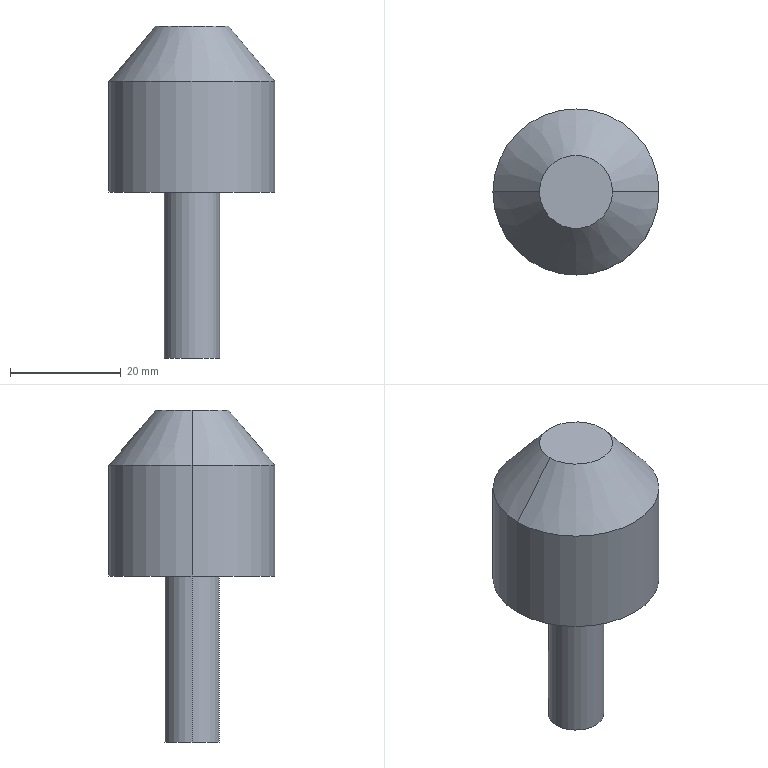Part | SolidWorks | features Chamfer 1, Extrusion 1, ICE 1 | 1 solid | 9 faces | box 30 x 30 x 60 mm | volume 20345 mm3 | cylinder 4 | plane 3 | cone 2 | commonest cylinder face diameters 10 x2 30 x2
STEP:
#1=CARTESIAN_POINT('',(6.609,0.,60.));
#2=VERTEX_POINT('',#1);
#3=CARTESIAN_POINT('',(-6.609,0.,60.));
#4=VERTEX_POINT('',#3);
#5=CARTESIAN_POINT('',(0.,0.,60.));
#6=DIRECTION('',(0.,0.,1.));
#7=DIRECTION('',(1.,0.,0.));
#8=AXIS2_PLACEMENT_3D('',#5,#6,#7);
#9=CIRCLE('',#8,6.609);
#10=EDGE_CURVE('',#2,#4,#9,.T.);
#11=ORIENTED_EDGE('',*,*,#10,.F.);
#12=CARTESIAN_POINT('',(15.,0.,50.));
#13=VERTEX_POINT('',#12);
#14=CARTESIAN_POINT('',(6.609,0.,60.));
#15=DIRECTION('',(0.6428,0.,-0.766));
#16=VECTOR('',#15,1000.);
#17=LINE('',#14,#16);
#18=EDGE_CURVE('',#2,#13,#17,.T.);
#19=ORIENTED_EDGE('',*,*,#18,.T.);
#20=CARTESIAN_POINT('',(-15.,0.,50.));
#21=VERTEX_POINT('',#20);
#22=CARTESIAN_POINT('',(0.,0.,50.));
#23=DIRECTION('',(0.,0.,-1.));
#24=DIRECTION('',(1.,0.,0.));
#25=AXIS2_PLACEMENT_3D('',#22,#23,#24);
#26=CIRCLE('',#25,15.);
#27=EDGE_CURVE('',#21,#13,#26,.T.);
#28=ORIENTED_EDGE('',*,*,#27,.F.);
#29=CARTESIAN_POINT('',(-6.609,0.,60.));
#30=DIRECTION('',(-0.6428,0.,-0.766));
#31=VECTOR('',#30,1000.);
#32=LINE('',#29,#31);
#33=EDGE_CURVE('',#4,#21,#32,.T.);
#34=ORIENTED_EDGE('',*,*,#33,.F.);
#35=EDGE_LOOP('',(#11,#19,#28,#34));
#36=FACE_OUTER_BOUND('',#35,.T.);
#37=CARTESIAN_POINT('',(0.,0.,60.));
#38=DIRECTION('',(0.,0.,-1.));
#39=DIRECTION('',(-1.,0.,0.));
#40=AXIS2_PLACEMENT_3D('',#37,#38,#39);
#41=CONICAL_SURFACE('',#40,6.609,0.6981);
#42=ADVANCED_FACE('',(#36),#41,.T.);
#43=ORIENTED_EDGE('',*,*,#27,.T.);
#44=CARTESIAN_POINT('',(15.,0.,30.));
#45=VERTEX_POINT('',#44);
#46=CARTESIAN_POINT('',(15.,0.,60.));
#47=DIRECTION('',(0.,0.,-1.));
#48=VECTOR('',#47,1000.);
#49=LINE('',#46,#48);
#50=EDGE_CURVE('',#13,#45,#49,.T.);
#51=ORIENTED_EDGE('',*,*,#50,.T.);
#52=CARTESIAN_POINT('',(-15.,0.,30.));
#53=VERTEX_POINT('',#52);
#54=CARTESIAN_POINT('',(0.,0.,30.));
#55=DIRECTION('',(0.,0.,1.));
#56=DIRECTION('',(1.,0.,0.));
#57=AXIS2_PLACEMENT_3D('',#54,#55,#56);
#58=CIRCLE('',#57,15.);
#59=EDGE_CURVE('',#45,#53,#58,.T.);
#60=ORIENTED_EDGE('',*,*,#59,.T.);
#61=CARTESIAN_POINT('',(-15.,0.,60.));
#62=DIRECTION('',(0.,0.,-1.));
#63=VECTOR('',#62,1000.);
#64=LINE('',#61,#63);
#65=EDGE_CURVE('',#21,#53,#64,.T.);
#66=ORIENTED_EDGE('',*,*,#65,.F.);
#67=EDGE_LOOP('',(#43,#51,#60,#66));
#68=FACE_OUTER_BOUND('',#67,.T.);
#69=CARTESIAN_POINT('',(0.,0.,60.));
#70=DIRECTION('',(0.,0.,-1.));
#71=DIRECTION('',(-1.,0.,0.));
#72=AXIS2_PLACEMENT_3D('',#69,#70,#71);
#73=CYLINDRICAL_SURFACE('',#72,15.);
#74=ADVANCED_FACE('',(#68),#73,.T.);
#75=CARTESIAN_POINT('',(5.,0.,30.));
#76=VERTEX_POINT('',#75);
#77=CARTESIAN_POINT('',(-5.,0.,30.));
#78=VERTEX_POINT('',#77);
#79=CARTESIAN_POINT('',(0.,0.,30.));
#80=DIRECTION('',(0.,0.,1.));
#81=DIRECTION('',(1.,0.,0.));
#82=AXIS2_PLACEMENT_3D('',#79,#80,#81);
#83=CIRCLE('',#82,5.);
#84=EDGE_CURVE('',#76,#78,#83,.T.);
#85=ORIENTED_EDGE('',*,*,#84,.F.);
#86=CARTESIAN_POINT('',(5.,0.,0.));
#87=VERTEX_POINT('',#86);
#88=CARTESIAN_POINT('',(5.,0.,30.));
#89=DIRECTION('',(0.,0.,-1.));
#90=VECTOR('',#89,1000.);
#91=LINE('',#88,#90);
#92=EDGE_CURVE('',#76,#87,#91,.T.);
#93=ORIENTED_EDGE('',*,*,#92,.T.);
#94=CARTESIAN_POINT('',(-5.,0.,0.));
#95=VERTEX_POINT('',#94);
#96=CARTESIAN_POINT('',(0.,0.,0.));
#97=DIRECTION('',(0.,0.,1.));
#98=DIRECTION('',(1.,0.,0.));
#99=AXIS2_PLACEMENT_3D('',#96,#97,#98);
#100=CIRCLE('',#99,5.);
#101=EDGE_CURVE('',#87,#95,#100,.T.);
#102=ORIENTED_EDGE('',*,*,#101,.T.);
#103=CARTESIAN_POINT('',(-5.,0.,30.));
#104=DIRECTION('',(0.,0.,-1.));
#105=VECTOR('',#104,1000.);
#106=LINE('',#103,#105);
#107=EDGE_CURVE('',#78,#95,#106,.T.);
#108=ORIENTED_EDGE('',*,*,#107,.F.);
#109=EDGE_LOOP('',(#85,#93,#102,#108));
#110=FACE_OUTER_BOUND('',#109,.T.);
#111=CARTESIAN_POINT('',(0.,0.,30.));
#112=DIRECTION('',(0.,0.,-1.));
#113=DIRECTION('',(-1.,0.,0.));
#114=AXIS2_PLACEMENT_3D('',#111,#112,#113);
#115=CYLINDRICAL_SURFACE('',#114,5.);
#116=ADVANCED_FACE('',(#110),#115,.T.);
#117=ORIENTED_EDGE('',*,*,#92,.F.);
#118=CARTESIAN_POINT('',(0.,0.,30.));
#119=DIRECTION('',(0.,0.,1.));
#120=DIRECTION('',(1.,0.,0.));
#121=AXIS2_PLACEMENT_3D('',#118,#119,#120);
#122=CIRCLE('',#121,5.);
#123=EDGE_CURVE('',#78,#76,#122,.T.);
#124=ORIENTED_EDGE('',*,*,#123,.F.);
#125=ORIENTED_EDGE('',*,*,#107,.T.);
#126=CARTESIAN_POINT('',(0.,0.,0.));
#127=DIRECTION('',(0.,0.,1.));
#128=DIRECTION('',(1.,0.,0.));
#129=AXIS2_PLACEMENT_3D('',#126,#127,#128);
#130=CIRCLE('',#129,5.);
#131=EDGE_CURVE('',#95,#87,#130,.T.);
#132=ORIENTED_EDGE('',*,*,#131,.T.);
#133=EDGE_LOOP('',(#117,#124,#125,#132));
#134=FACE_OUTER_BOUND('',#133,.T.);
#135=CARTESIAN_POINT('',(0.,0.,30.));
#136=DIRECTION('',(0.,0.,-1.));
#137=DIRECTION('',(-1.,0.,0.));
#138=AXIS2_PLACEMENT_3D('',#135,#136,#137);
#139=CYLINDRICAL_SURFACE('',#138,5.);
#140=ADVANCED_FACE('',(#134),#139,.T.);
#141=ORIENTED_EDGE('',*,*,#131,.F.);
#142=ORIENTED_EDGE('',*,*,#101,.F.);
#143=EDGE_LOOP('',(#141,#142));
#144=FACE_OUTER_BOUND('',#143,.T.);
#145=CARTESIAN_POINT('',(0.,0.,0.));
#146=DIRECTION('',(0.,0.,1.));
#147=DIRECTION('',(1.,0.,0.));
#148=AXIS2_PLACEMENT_3D('',#145,#146,#147);
#149=PLANE('',#148);
#150=ADVANCED_FACE('',(#144),#149,.F.);
#151=CARTESIAN_POINT('',(0.,0.,30.));
#152=DIRECTION('',(0.,0.,1.));
#153=DIRECTION('',(1.,0.,0.));
#154=AXIS2_PLACEMENT_3D('',#151,#152,#153);
#155=CIRCLE('',#154,15.);
#156=EDGE_CURVE('',#53,#45,#155,.T.);
#157=ORIENTED_EDGE('',*,*,#156,.F.);
#158=ORIENTED_EDGE('',*,*,#59,.F.);
#159=EDGE_LOOP('',(#157,#158));
#160=FACE_OUTER_BOUND('',#159,.T.);
#161=ORIENTED_EDGE('',*,*,#123,.T.);
#162=ORIENTED_EDGE('',*,*,#84,.T.);
#163=EDGE_LOOP('',(#161,#162));
#164=FACE_BOUND('',#163,.T.);
#165=CARTESIAN_POINT('',(0.,0.,30.));
#166=DIRECTION('',(0.,0.,1.));
#167=DIRECTION('',(1.,0.,0.));
#168=AXIS2_PLACEMENT_3D('',#165,#166,#167);
#169=PLANE('',#168);
#170=ADVANCED_FACE('',(#160,#164),#169,.F.);
#171=ORIENTED_EDGE('',*,*,#50,.F.);
#172=CARTESIAN_POINT('',(0.,0.,50.));
#173=DIRECTION('',(0.,0.,-1.));
#174=DIRECTION('',(1.,0.,0.));
#175=AXIS2_PLACEMENT_3D('',#172,#173,#174);
#176=CIRCLE('',#175,15.);
#177=EDGE_CURVE('',#13,#21,#176,.T.);
#178=ORIENTED_EDGE('',*,*,#177,.T.);
#179=ORIENTED_EDGE('',*,*,#65,.T.);
#180=ORIENTED_EDGE('',*,*,#156,.T.);
#181=EDGE_LOOP('',(#171,#178,#179,#180));
#182=FACE_OUTER_BOUND('',#181,.T.);
#183=CARTESIAN_POINT('',(0.,0.,60.));
#184=DIRECTION('',(0.,0.,-1.));
#185=DIRECTION('',(-1.,0.,0.));
#186=AXIS2_PLACEMENT_3D('',#183,#184,#185);
#187=CYLINDRICAL_SURFACE('',#186,15.);
#188=ADVANCED_FACE('',(#182),#187,.T.);
#189=CARTESIAN_POINT('',(0.,0.,60.));
#190=DIRECTION('',(0.,0.,1.));
#191=DIRECTION('',(1.,0.,0.));
#192=AXIS2_PLACEMENT_3D('',#189,#190,#191);
#193=CIRCLE('',#192,6.609);
#194=EDGE_CURVE('',#4,#2,#193,.T.);
#195=ORIENTED_EDGE('',*,*,#194,.T.);
#196=ORIENTED_EDGE('',*,*,#10,.T.);
#197=EDGE_LOOP('',(#195,#196));
#198=FACE_OUTER_BOUND('',#197,.T.);
#199=CARTESIAN_POINT('',(0.,0.,60.));
#200=DIRECTION('',(0.,0.,1.));
#201=DIRECTION('',(1.,0.,0.));
#202=AXIS2_PLACEMENT_3D('',#199,#200,#201);
#203=PLANE('',#202);
#204=ADVANCED_FACE('',(#198),#203,.T.);
#205=ORIENTED_EDGE('',*,*,#18,.F.);
#206=ORIENTED_EDGE('',*,*,#194,.F.);
#207=ORIENTED_EDGE('',*,*,#33,.T.);
#208=ORIENTED_EDGE('',*,*,#177,.F.);
#209=EDGE_LOOP('',(#205,#206,#207,#208));
#210=FACE_OUTER_BOUND('',#209,.T.);
#211=CARTESIAN_POINT('',(0.,0.,60.));
#212=DIRECTION('',(0.,0.,-1.));
#213=DIRECTION('',(-1.,0.,0.));
#214=AXIS2_PLACEMENT_3D('',#211,#212,#213);
#215=CONICAL_SURFACE('',#214,6.609,0.6981);
#216=ADVANCED_FACE('',(#210),#215,.T.);
#217=CLOSED_SHELL('',(#42,#74,#116,#140,#150,#170,#188,#204,#216));
#218=MANIFOLD_SOLID_BREP('',#217);
#219=CARTESIAN_POINT('',(0.,0.,0.));
#220=DIRECTION('',(0.,0.,1.));
#221=DIRECTION('',(1.,0.,0.));
#222=AXIS2_PLACEMENT_3D('',#219,#220,#221);
#223=(LENGTH_UNIT()NAMED_UNIT(*)SI_UNIT(.MILLI.,.METRE.));
#224=UNCERTAINTY_MEASURE_WITH_UNIT(LENGTH_MEASURE(0.00001),#223,'','');
#225=(NAMED_UNIT(*)PLANE_ANGLE_UNIT()SI_UNIT($,.RADIAN.));
#226=(NAMED_UNIT(*)SI_UNIT($,.STERADIAN.)SOLID_ANGLE_UNIT());
#227=(GEOMETRIC_REPRESENTATION_CONTEXT(3)GLOBAL_UNCERTAINTY_ASSIGNED_CONTEXT((#224))GLOBAL_UNIT_ASSIGNED_CONTEXT((#223,#225,#226))REPRESENTATION_CONTEXT('',''));
#228=ADVANCED_BREP_SHAPE_REPRESENTATION('',(#218,#222),#227);